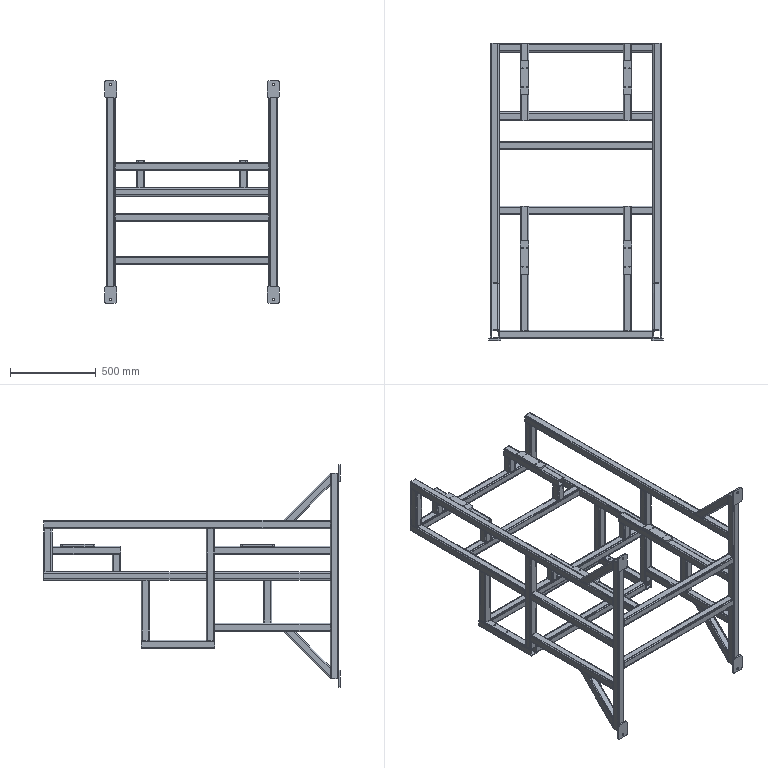Part | SolidWorks | features MirrorSolid 7, WeldCornerFeat 7, ICE 3, MoveCopyBody 3, Fillet 2, WeldMemberFeat 2, 3DProfileFeature 1, Cut 1, EndCap 1, Gusset 1, HoleWzd 1, LPattern 1, MirrorPattern 1, WeldmentFeature 1 | 49 solids | 886 faces | box 1020 x 1735 x 1300 mm | volume 17820263 mm3 | plane 470 | cylinder 416 | commonest cylinder face diameters 8 x176 16 x160 6.8 x40 20 x32 14 x8